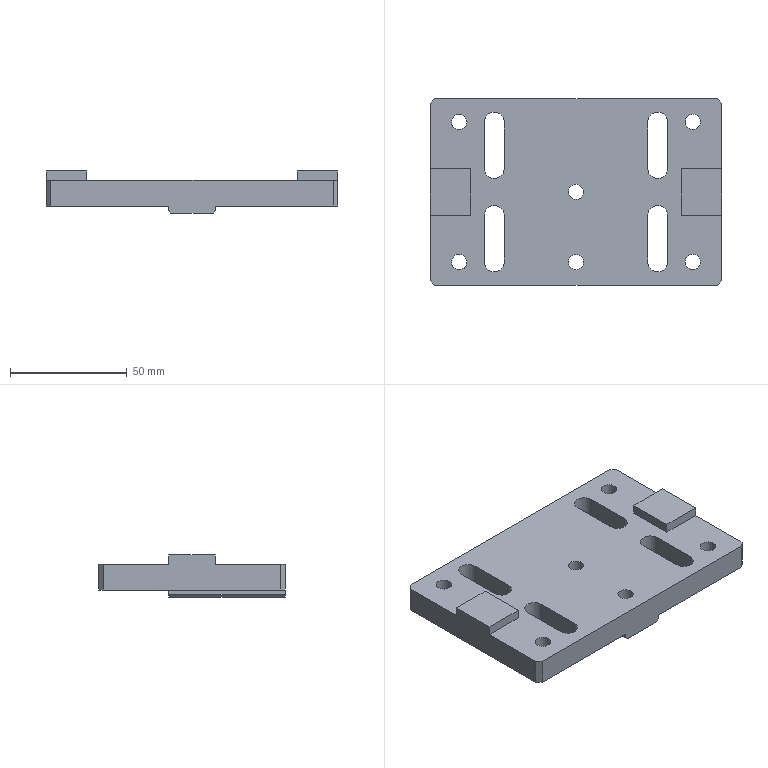NC program | NX | posted with a generic post | part box 125 x 80 x 18 mm
Whole program:
N10 G17 G21 G94 G90
(FLOOR_WALL_COPY , TOOL : D63)
N12 T01 M6
N14 G54
N16 G17 G0 G90 X39.997 Y97. S6500 M3
N18 G43 Z30. H1
N20 Z4.
N22 G94 G1 Z1. F1500.
N24 Y94.
N26 Y-94.
N28 X12.599
N30 Y94.
N32 X-14.8
N34 Y-94.
N36 Y-97.
N38 Z4.
N40 G0 Z30.
N42 X39.997 Y97.
N44 Z3.
N46 G1 Z0.
N48 Y94.
N50 Y-94.
N52 X12.599
N54 Y94.
N56 X-14.8
N58 Y-94.
N60 Y-97.
N62 Z3.
N64 G0 Z30.
N66 M5
(FLOOR_WALL_1_COPY_1 , TOOL : D10)
N68 T04 M6
N70 G54
N72 G17 G0 G90 X-46.5 Y-1. S7000 M3
N74 G43 Z30. H4
N76 Z0.525
N78 G94 G1 Z-0.975 F1000.
N80 X-41.
N82 G3 X-40. Y0. R1.
N84 G1 Y60.5 F3000.
N86 X-38. Y62.5
N88 X-15.1
N90 Y39.9
N92 X15.1
N94 Y62.5
N96 X38.
N98 X40. Y60.5
N100 Y-60.5
N102 X38. Y-62.5
N104 X15.1
N106 Y-55.5
N108 Y-39.9
N110 X-15.1
N112 Y-62.5
N114 X-38.
N116 X-40. Y-60.5
N118 Y0.
N120 X-33.
N122 Y55.5
N124 X-22.1
N126 Y39.9
N128 G3 X-15.1 Y32.9 R7.
N130 G1 X15.1
N132 G3 X22.1 Y39.9 R7.
N134 G1 Y55.5
N136 X33.
N138 Y-55.5
N140 X22.1
N142 Y-39.9
N144 G3 X15.1 Y-32.9 R7.
N146 G1 X-15.1
N148 G3 X-22.1 Y-39.9 R7.
N150 G1 Y-55.5
N152 X-33.
N154 Y0.
N156 X-26.
N158 Y31.114
N160 X-26.479 Y36.091
N162 G2 X-27.1 Y39.9 R12.
N164 G1 Y50.5
N166 X-28.
N168 Y35.697
N170 G2 X-26.479 Y36.091 R5.
N172 G1 X-26. Y31.114
N174 G3 X-15.1 Y25.9 R14.
N176 G1 X15.1
N178 G3 X26. Y31.114 R14.
N180 G1 X28. Y35.697
N182 Y50.5
N184 X27.1
N186 Y39.9
N188 G2 X26.479 Y36.091 R12.
N190 X28. Y35.697 R5.
N192 G1 X26. Y31.114
N194 Y-31.114
N196 X26.479 Y-36.091
N198 G2 X27.1 Y-39.9 R12.
N200 G1 Y-50.5
N202 X28.
N204 Y-35.697
N206 G2 X26.479 Y-36.091 R5.
N208 G1 X26. Y-31.114
N210 G3 X15.1 Y-25.9 R14.
N212 G1 X-15.1
N214 G3 X-26. Y-31.114 R14.
N216 G1 X-28. Y-35.697
N218 Y-50.5
N220 X-27.1
N222 Y-39.9
N224 G2 X-26.479 Y-36.091 R12.
N226 X-28. Y-35.697 R5.
N228 G1 X-26. Y-31.114
N230 Y0.
N232 X-19.
N234 Y19.265
N236 G3 X-15.1 Y18.9 R21.
N238 G1 X15.1
N240 G3 X19. Y19.265 R21.
N242 G1 Y-19.265
N244 G3 X15.1 Y-18.9 R21.
N246 G1 X-15.1
N248 G3 X-19. Y-19.265 R21.
N250 G1 Y0.
N252 X-12.
N254 Y11.9
N256 X12.
N258 Y-11.9
N260 X-12.
N262 Y0.
N264 X-5.
N266 Y4.9
N268 X5.
N270 Y-4.9
N272 X-5.
N274 Y0.
N276 X-0.5
N278 Y0.4
N280 X0.5
N282 Y-0.4
N284 X-0.5
N286 Y0.
N288 G3 X-1.5 Y1. R1.
N290 G1 Z0.525
N292 G0 X-46.5 Y-1. Z-0.45
N294 G1 Z-1.95 F1000.
N296 X-41.
N298 G3 X-40. Y0. R1.
N300 G1 Y60.5 F3000.
N302 X-38. Y62.5
N304 X-15.1
N306 Y39.9
N308 X15.1
N310 Y62.5
N312 X38.
N314 X40. Y60.5
N316 Y-60.5
N318 X38. Y-62.5
N320 X15.1
N322 Y-55.5
N324 Y-39.9
N326 X-15.1
N328 Y-62.5
N330 X-38.
N332 X-40. Y-60.5
N334 Y0.
N336 X-33.
N338 Y55.5
N340 X-22.1
N342 Y39.9
N344 G3 X-15.1 Y32.9 R7.
N346 G1 X15.1
N348 G3 X22.1 Y39.9 R7.
N350 G1 Y55.5
N352 X33.
N354 Y-55.5
N356 X22.1
N358 Y-39.9
N360 G3 X15.1 Y-32.9 R7.
N362 G1 X-15.1
N364 G3 X-22.1 Y-39.9 R7.
N366 G1 Y-55.5
N368 X-33.
N370 Y0.
N372 X-26.
N374 Y31.114
N376 X-26.479 Y36.091
N378 G2 X-27.1 Y39.9 R12.
N380 G1 Y50.5
N382 X-28.
N384 Y35.697
N386 G2 X-26.479 Y36.091 R5.
N388 G1 X-26. Y31.114
N390 G3 X-15.1 Y25.9 R14.
N392 G1 X15.1
N394 G3 X26. Y31.114 R14.
N396 G1 X28. Y35.697
N398 Y50.5
N400 X27.1
N402 Y39.9
N404 G2 X26.479 Y36.091 R12.
N406 X28. Y35.697 R5.
N408 G1 X26. Y31.114
N410 Y-31.114
N412 X26.479 Y-36.091
N414 G2 X27.1 Y-39.9 R12.
N416 G1 Y-50.5
N418 X28.
N420 Y-35.697
N422 G2 X26.479 Y-36.091 R5.
N424 G1 X26. Y-31.114
N426 G3 X15.1 Y-25.9 R14.
N428 G1 X-15.1
N430 G3 X-26. Y-31.114 R14.
N432 G1 X-28. Y-35.697
N434 Y-50.5
N436 X-27.1
N438 Y-39.9
N440 G2 X-26.479 Y-36.091 R12.
N442 X-28. Y-35.697 R5.
N444 G1 X-26. Y-31.114
N446 Y0.
N448 X-19.
N450 Y19.265
N452 G3 X-15.1 Y18.9 R21.
N454 G1 X15.1
N456 G3 X19. Y19.265 R21.
N458 G1 Y-19.265
N460 G3 X15.1 Y-18.9 R21.
N462 G1 X-15.1
N464 G3 X-19. Y-19.265 R21.
N466 G1 Y0.
N468 X-12.
N470 Y11.9
N472 X12.
N474 Y-11.9
N476 X-12.
N478 Y0.
N480 X-5.
N482 Y4.9
N484 X5.
N486 Y-4.9
N488 X-5.
N490 Y0.
N492 X-0.5
N494 Y0.4
N496 X0.5
N498 Y-0.4
N500 X-0.5
N502 Y0.
N504 G3 X-1.5 Y1. R1.
N506 G1 Z-0.45
N508 G0 X-46.5 Y-1. Z-1.425
N510 G1 Z-2.925 F1000.
N512 X-41.
N514 G3 X-40. Y0. R1.
N516 G1 Y60.5 F3000.
N518 X-38. Y62.5
N520 X-15.1
N522 Y39.9
N524 X15.1
N526 Y62.5
N528 X38.
N530 X40. Y60.5
N532 Y-60.5
N534 X38. Y-62.5
N536 X15.1
N538 Y-55.5
N540 Y-39.9
N542 X-15.1
N544 Y-62.5
N546 X-38.
N548 X-40. Y-60.5
N550 Y0.
N552 X-33.
N554 Y55.5
N556 X-22.1
N558 Y39.9
N560 G3 X-15.1 Y32.9 R7.
N562 G1 X15.1
N564 G3 X22.1 Y39.9 R7.
N566 G1 Y55.5
N568 X33.
N570 Y-55.5
N572 X22.1
N574 Y-39.9
N576 G3 X15.1 Y-32.9 R7.
N578 G1 X-15.1
N580 G3 X-22.1 Y-39.9 R7.
N582 G1 Y-55.5
N584 X-33.
N586 Y0.
N588 X-26.
N590 Y31.114
N592 X-26.479 Y36.091
N594 G2 X-27.1 Y39.9 R12.
N596 G1 Y50.5
N598 X-28.
N600 Y35.697
N602 G2 X-26.479 Y36.091 R5.
N604 G1 X-26. Y31.114
N606 G3 X-15.1 Y25.9 R14.
N608 G1 X15.1
N610 G3 X26. Y31.114 R14.
N612 G1 X28. Y35.697
N614 Y50.5
N616 X27.1
N618 Y39.9
N620 G2 X26.479 Y36.091 R12.
N622 X28. Y35.697 R5.
N624 G1 X26. Y31.114
N626 Y-31.114
N628 X26.479 Y-36.091
N630 G2 X27.1 Y-39.9 R12.
N632 G1 Y-50.5
N634 X28.
N636 Y-35.697
N638 G2 X26.479 Y-36.091 R5.
N640 G1 X26. Y-31.114
N642 G3 X15.1 Y-25.9 R14.
N644 G1 X-15.1
N646 G3 X-26. Y-31.114 R14.
N648 G1 X-28. Y-35.697
N650 Y-50.5
N652 X-27.1
N654 Y-39.9
N656 G2 X-26.479 Y-36.091 R12.
N658 X-28. Y-35.697 R5.
N660 G1 X-26. Y-31.114
N662 Y0.
N664 X-19.
N666 Y19.265
N668 G3 X-15.1 Y18.9 R21.
N670 G1 X15.1
N672 G3 X19. Y19.265 R21.
N674 G1 Y-19.265
N676 G3 X15.1 Y-18.9 R21.
N678 G1 X-15.1
N680 G3 X-19. Y-19.265 R21.
N682 G1 Y0.
N684 X-12.
N686 Y11.9
N688 X12.
N690 Y-11.9
N692 X-12.
N694 Y0.
N696 X-5.
N698 Y4.9
N700 X5.
N702 Y-4.9
N704 X-5.
N706 Y0.
N708 X-0.5
N710 Y0.4
N712 X0.5
N714 Y-0.4
N716 X-0.5
N718 Y0.
N720 G3 X-1.5 Y1. R1.
N722 G1 Z-1.425
N724 G0 X-46.5 Y-1. Z-2.4
N726 G1 Z-3.9 F1000.
N728 X-41.
N730 G3 X-40. Y0. R1.
N732 G1 Y60.5 F3000.
N734 X-38. Y62.5
N736 X-15.1
N738 Y39.9
N740 X15.1
N742 Y62.5
N744 X38.
N746 X40. Y60.5
N748 Y-60.5
N750 X38. Y-62.5
N752 X15.1
N754 Y-55.5
N756 Y-39.9
N758 X-15.1
N760 Y-62.5
N762 X-38.
N764 X-40. Y-60.5
N766 Y0.
N768 X-33.
N770 Y55.5
N772 X-22.1
N774 Y39.9
N776 G3 X-15.1 Y32.9 R7.
N778 G1 X15.1
N780 G3 X22.1 Y39.9 R7.
N782 G1 Y55.5
N784 X33.
N786 Y-55.5
N788 X22.1
N790 Y-39.9
N792 G3 X15.1 Y-32.9 R7.
N794 G1 X-15.1
N796 G3 X-22.1 Y-39.9 R7.
N798 G1 Y-55.5
N800 X-33.
N802 Y0.
N804 X-26.
N806 Y31.114
N808 X-26.479 Y36.091
N810 G2 X-27.1 Y39.9 R12.
N812 G1 Y50.5
N814 X-28.
N816 Y35.697
N818 G2 X-26.479 Y36.091 R5.
N820 G1 X-26. Y31.114
N822 G3 X-15.1 Y25.9 R14.
N824 G1 X15.1
N826 G3 X26. Y31.114 R14.
N828 G1 X28. Y35.697
N830 Y50.5
N832 X27.1
N834 Y39.9
N836 G2 X26.479 Y36.091 R12.
N838 X28. Y35.697 R5.
N840 G1 X26. Y31.114
N842 Y-31.114
N844 X26.479 Y-36.091
N846 G2 X27.1 Y-39.9 R12.
N848 G1 Y-50.5
N850 X28.
N852 Y-35.697
N854 G2 X26.479 Y-36.091 R5.
N856 G1 X26. Y-31.114
N858 G3 X15.1 Y-25.9 R14.
N860 G1 X-15.1
N862 G3 X-26. Y-31.114 R14.
N864 G1 X-28. Y-35.697
N866 Y-50.5
N868 X-27.1
N870 Y-39.9
N872 G2 X-26.479 Y-36.091 R12.
N874 X-28. Y-35.697 R5.
N876 G1 X-26. Y-31.114
N878 Y0.
N880 X-19.
N882 Y19.265
N884 G3 X-15.1 Y18.9 R21.
N886 G1 X15.1
N888 G3 X19. Y19.265 R21.
N890 G1 Y-19.265
N892 G3 X15.1 Y-18.9 R21.
N894 G1 X-15.1
N896 G3 X-19. Y-19.265 R21.
N898 G1 Y0.
N900 X-12.
N902 Y11.9
N904 X12.
N906 Y-11.9
N908 X-12.
N910 Y0.
N912 X-5.
N914 Y4.9
N916 X5.
N918 Y-4.9
N920 X-5.
N922 Y0.
N924 X-0.5
N926 Y0.4
N928 X0.5
N930 Y-0.4
N932 X-0.5
N934 Y0.
N936 G3 X-1.5 Y1. R1.
N938 G1 Z-2.4
N940 G0 Z30.
(FLOOR_WALL_1_COPY_COPY , TOOL : D10)
N942 X-46. Y63.692
N944 Z-2.5
N946 G1 Z-4. F1000.
N948 Y63.497
N950 G3 X-45. Y62.497 R1.
N952 G1 X-15.5 F1200.
N954 Y57.657
N956 X-45.
N958 Y52.817
N960 X-15.5
N962 Y47.977
N964 X-45.
N966 Y43.137
N968 X-15.5
N970 G3 X-16.5 Y44.137 R1.
N972 G1 Z-2.5
N974 G0 Z30.
N976 X6.17 Y69.
N978 Z-1.5
N980 G1 X15.5 Z-4. F1000.
N982 Y62.497
N984 X45. F1200.
N986 Y57.657
N988 X15.5
N990 Y52.817
N992 X45.
N994 Y47.977
N996 X15.5
N998 Y43.137
N1000 X45.
N1002 Y38.298
N1004 X-45.
N1006 Y33.458
N1008 X45.
N1010 Y28.618
N1012 X-45.
N1014 Y23.778
N1016 X45.
N1018 Y18.938
N1020 X-45.
N1022 Y14.098
N1024 X45.
N1026 Y9.258
N1028 X-45.
N1030 Y4.418
N1032 X45.
N1034 Y-0.421
N1036 X-45.
N1038 Y-5.261
N1040 X45.
N1042 Y-10.101
N1044 X-45.
N1046 Y-14.941
N1048 X45.
N1050 Y-19.781
N1052 X-45.
N1054 Y-24.621
N1056 X45.
N1058 Y-29.461
N1060 X-45.
N1062 Y-34.301
N1064 X45.
N1066 Y-39.14
N1068 X-45.
N1070 Y-43.98
N1072 X-15.5
N1074 Y-48.82
N1076 X-45.
N1078 Y-53.66
N1080 X-15.5
N1082 Y-58.5
N1084 X-45.
N1086 Y-62.571
N1088 X-44.231 Y-63.34
N1090 X-15.5
N1092 G3 X-16.5 Y-62.34 R1.
N1094 G1 Z-2.5
N1096 G0 Z0.
N1098 G1 X-15.5 Y-43.98 F8000.
N1100 G0 Z-2.5
N1102 G1 Z-4. F1000.
N1104 Y-40.
N1106 G2 X-15. Y-39.5 R0.5
N1108 G1 X15.
N1110 G2 X15.5 Y-40. R0.5
N1112 G1 Y-43.98
N1114 X45. F1200.
N1116 Y-48.82
N1118 X15.5
N1120 Y-53.66
N1122 X45.
N1124 Y-58.5
N1126 X15.5
N1128 Y-63.34
N1130 X44.231
N1132 G3 X45.231 Y-62.34 R1.
N1134 G1 X46.5
N1136 Z-2.5
N1138 G0 Z30.
N1140 X-16. Y-69.
N1142 Z-2.5
N1144 G1 Z-4. F1000.
N1146 Y-68.5
N1148 G3 X-15. Y-67.5 R1.
N1150 G1 Y-40. F1200.
N1152 X15.
N1154 Y-67.5
N1156 G3 X16. Y-68.5 R1.
N1158 G1 Y-69.
N1160 Z-2.5
N1162 G0 Z0.
N1164 G1 Y69. F8000.
N1166 G0 Z-2.5
N1168 G1 Z-4. F1000.
N1170 Y68.5
N1172 G3 X15. Y67.5 R1.
N1174 G1 Y40. F1200.
N1176 X-15.
N1178 Y67.5
N1180 G3 X-16. Y68.5 R1.
N1182 G1 Y69.
N1184 Z-2.5
N1186 G0 Z30.
N1188 M5
(PLANAR_MILL_COPY_COPY_COPY , TOOL : D8A45)
N1190 T06 M6
N1192 G54
N1194 G17 G0 G90 X1.501 Y-65.5 S7000 M3
N1196 G43 Z30. H6
N1198 Z0.
N1200 G94 G1 Z-1.5 F1250.
N1202 X0.866 Y-64.4
N1204 G3 X0. Y-63.9 R1.
N1206 G1 X-9.9
N1208 G2 X-11.4 Y-62.4 R1.5
N1210 G1 Y-45.1
N1212 G2 X-9.9 Y-43.6 R1.5
N1214 G1 X9.9
N1216 G2 X11.4 Y-45.1 R1.5
N1218 G1 Y-62.4
N1220 G2 X9.9 Y-63.9 R1.5
N1222 G1 X0.
N1224 G3 X-0.866 Y-64.4 R1.
N1226 G1 X-1.501 Y-65.5
N1228 Z0.
N1230 G0 Z30.
N1232 Y65.5
N1234 Z0.
N1236 G1 Z-1.5
N1238 X-0.866 Y64.4
N1240 G3 X0. Y63.9 R1.
N1242 G1 X9.9
N1244 G2 X11.4 Y62.4 R1.5
N1246 G1 Y45.1
N1248 G2 X9.9 Y43.6 R1.5
N1250 G1 X-9.9
N1252 G2 X-11.4 Y45.1 R1.5
N1254 G1 Y62.4
N1256 G2 X-9.9 Y63.9 R1.5
N1258 G1 X0.
N1260 G3 X0.866 Y64.4 R1.
N1262 G1 X1.501 Y65.5
N1264 Z0.
N1266 G0 Z30.
(PLANAR_MILL_COPY_COPY_COPY_COPY , TOOL : D8A45)
N1268 X30.255 Y-50.158
N1270 Z-4.
N1272 G1 Z-5.5
N1274 X31.4 Y-50.866
N1276 G3 X31.9 Y-50. R1.
N1278 X30. Y-48.1 R1.9
N1280 X31.9 Y-50. R-1.9
N1282 X31.4 Y-49.134 R1.
N1284 G1 X30.255 Y-49.842
N1286 Z-4.
N1288 G0 Z30.
N1290 X18.499 Y-36.25
N1292 Z-4.
N1294 G1 Z-5.5
N1296 X19.134 Y-37.35
N1298 G3 X20. Y-37.85 R1.
N1300 G1 X30.
N1302 G3 X32.85 Y-35. R2.85
N1304 X30. Y-32.15 R2.85
N1306 G1 X10.
N1308 G3 X7.15 Y-35. R2.85
N1310 X10. Y-37.85 R2.85
N1312 G1 X20.
N1314 G3 X20.866 Y-37.35 R1.
N1316 G1 X21.501 Y-36.25
N1318 Z-4.
N1320 G0 Z30.
N1322 X-30.255 Y-49.842
N1324 Z-4.
N1326 G1 Z-5.5
N1328 X-31.4 Y-49.134
N1330 G3 X-31.9 Y-50. R1.
N1332 X-30. Y-51.9 R1.9
N1334 X-31.9 Y-50. R-1.9
N1336 X-31.4 Y-50.866 R1.
N1338 G1 X-30.255 Y-50.158
N1340 Z-4.
N1342 G0 Z30.
N1344 X-21.501 Y-36.25
N1346 Z-4.
N1348 G1 Z-5.5
N1350 X-20.866 Y-37.35
N1352 G3 X-20. Y-37.85 R1.
N1354 G1 X-10.
N1356 G3 X-7.15 Y-35. R2.85
N1358 X-10. Y-32.15 R2.85
N1360 G1 X-30.
N1362 G3 X-32.85 Y-35. R2.85
N1364 X-30. Y-37.85 R2.85
N1366 G1 X-20.
N1368 G3 X-19.134 Y-37.35 R1.
N1370 G1 X-18.499 Y-36.25
N1372 Z-4.
N1374 G0 Z30.
N1376 X-15.204 Y-65.683
N1378 Z-4.
N1380 G1 Z-5.5
N1382 X-14.482 Y-64.879
N1384 G3 X-14.277 Y-63.9 R1.
N1386 G1 X-37.959
N1388 G2 X-39.019 Y-63.461 R1.5
N1390 G1 X-40.961 Y-61.519
N1392 G2 X-41.4 Y-60.459 R1.5
N1394 G1 Y60.459
N1396 G2 X-40.961 Y61.519 R1.5
N1398 G1 X-39.019 Y63.461
N1400 G2 X-37.959 Y63.9 R1.5
N1402 G1 X-14.277
N1404 G3 X-14.482 Y64.879 R1.
N1406 G1 X-15.204 Y65.683
N1408 Z-4.
N1410 G0 Z30.
N1412 X15.204
N1414 Z-4.
N1416 G1 Z-5.5
N1418 X14.482 Y64.879
N1420 G3 X14.277 Y63.9 R1.
N1422 G1 X37.959
N1424 G2 X39.019 Y63.461 R1.5
N1426 G1 X40.961 Y61.519
N1428 G2 X41.4 Y60.459 R1.5
N1430 G1 Y-60.459
N1432 G2 X40.961 Y-61.519 R1.5
N1434 G1 X39.019 Y-63.461
N1436 G2 X37.959 Y-63.9 R1.5
N1438 G1 X14.277
N1440 G3 X14.482 Y-64.879 R1.
N1442 G1 X15.204 Y-65.683
N1444 Z-4.
N1446 G0 Z30.
N1448 X-0.21 Y0.135
N1450 Z-4.
N1452 G1 Z-5.5
N1454 X-1.35 Y0.866
N1456 G3 X-1.85 Y0. R1.
N1458 X0. Y-1.85 R1.85
N1460 X-1.85 Y0. R-1.85
N1462 X-1.35 Y-0.866 R1.
N1464 G1 X-0.21 Y-0.135
N1466 Z-4.
N1468 G0 Z30.
N1470 X-30.21 Y0.135
N1472 Z-4.
N1474 G1 Z-5.5
N1476 X-31.35 Y0.866
N1478 G3 X-31.85 Y0. R1.
N1480 X-30. Y-1.85 R1.85
N1482 X-31.85 Y0. R-1.85
N1484 X-31.35 Y-0.866 R1.
N1486 G1 X-30.21 Y-0.135
N1488 Z-4.
N1490 G0 Z30.
N1492 X-21.501 Y33.75
N1494 Z-4.
N1496 G1 Z-5.5
N1498 X-20.866 Y32.65
N1500 G3 X-20. Y32.15 R1.
N1502 G1 X-10.
N1504 G3 X-7.15 Y35. R2.85
N1506 X-10. Y37.85 R2.85
N1508 G1 X-30.
N1510 G3 X-32.85 Y35. R2.85
N1512 X-30. Y32.15 R2.85
N1514 G1 X-20.
N1516 G3 X-19.134 Y32.65 R1.
N1518 G1 X-18.499 Y33.75
N1520 Z-4.
N1522 G0 Z30.
N1524 X-30.255 Y50.158
N1526 Z-4.
N1528 G1 Z-5.5
N1530 X-31.4 Y50.866
N1532 G3 X-31.9 Y50. R1.
N1534 X-30. Y48.1 R1.9
N1536 X-31.9 Y50. R-1.9
N1538 X-31.4 Y49.134 R1.
N1540 G1 X-30.255 Y49.842
N1542 Z-4.
N1544 G0 Z30.
N1546 X21.501 Y36.25
N1548 Z-4.
N1550 G1 Z-5.5
N1552 X20.866 Y37.35
N1554 G3 X20. Y37.85 R1.
N1556 G1 X10.
N1558 G3 X7.15 Y35. R2.85
N1560 X10. Y32.15 R2.85
N1562 G1 X30.
N1564 G3 X32.85 Y35. R2.85
N1566 X30. Y37.85 R2.85
N1568 G1 X20.
N1570 G3 X19.134 Y37.35 R1.
N1572 G1 X18.499 Y36.25
N1574 Z-4.
N1576 G0 Z30.
N1578 X30.255 Y49.842
N1580 Z-4.
N1582 G1 Z-5.5
N1584 X31.4 Y49.134
N1586 G3 X31.9 Y50. R1.
N1588 X30. Y51.9 R1.9
N1590 X31.9 Y50. R-1.9
N1592 X31.4 Y50.866 R1.
N1594 G1 X30.255 Y50.158
N1596 Z-4.
N1598 G0 Z30.
N1600 M5
N1602 M2